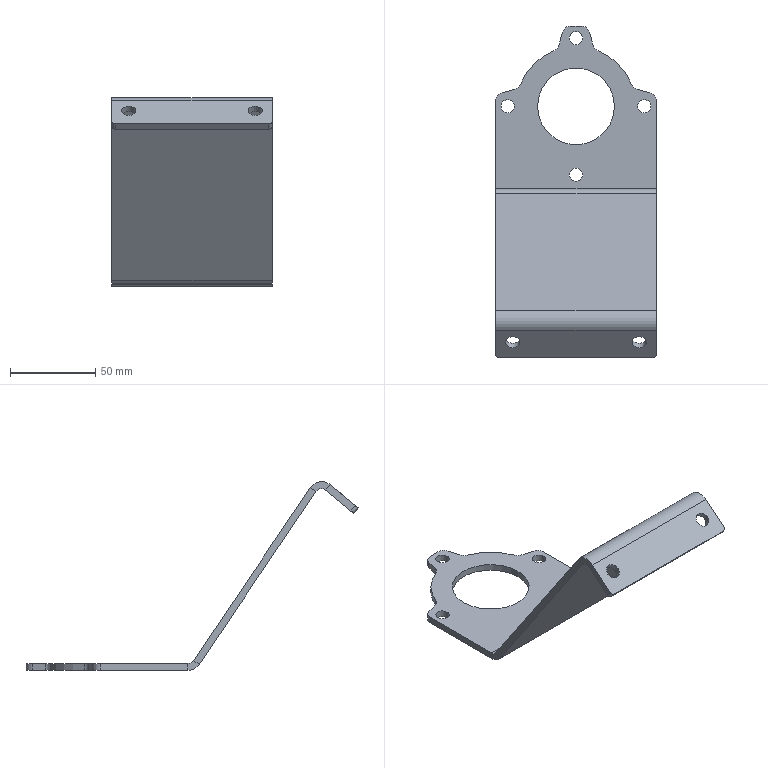Part | STEP file | Support gearmotor part2 B | 1 solid | 45 faces | box 94 x 194.451 x 110.566 mm | volume 79699 mm3 | cylinder 23 | plane 22 | commonest cylinder face diameters 10 x8 7.8 x4 4 x2 8 x2 8.3 x2 16 x2